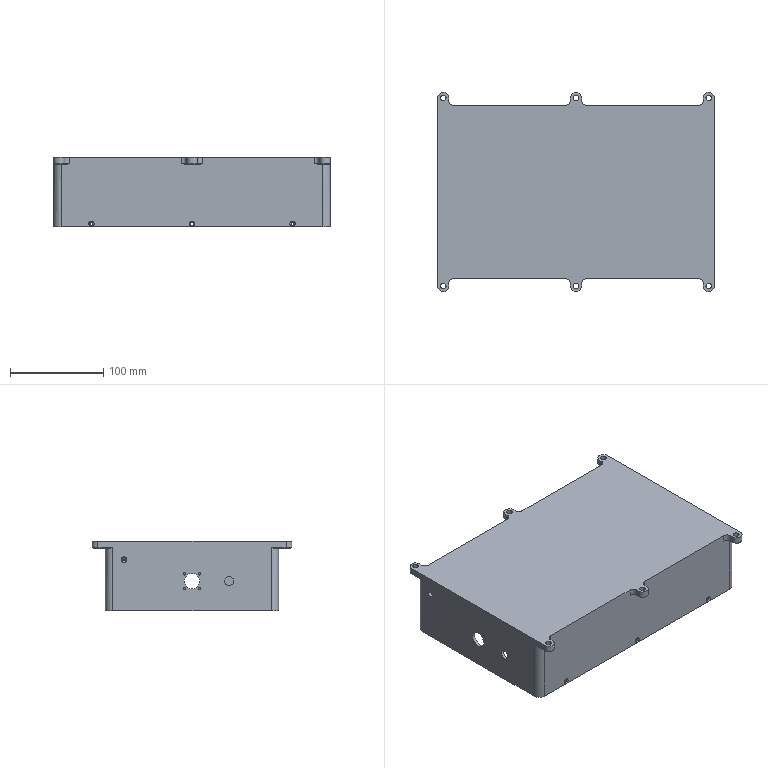NC program | NX | posted with a generic post | part box 297 x 214 x 75 mm
Whole program:
N10 G17 G21 G94 G90
(FLOOR_WALL_1_COPY_COPY , TOOL : D16)
N12 T02 M6
N14 G54
N16 G17 G0 G90 X-159.5 Y83.061 B0. C0. S7500 M3
N18 G43 Z30. H2
N20 Z-65.5
N22 G94 G1 Z-67. F1000.
N24 X-157.338 Y84.209
N26 G3 X-156.49 Y85.566 R1.6
N28 G2 X-140.5 Y101. R16.
N30 G1 X-128.5
N32 G3 X-127.114 Y101.8 R1.6
N34 G1 X-125.844 Y104.
N36 Z-65.5
N38 G0 Z30.
N40 X-16.656
N42 Z-65.5
N44 G1 Z-67.
N46 X-15.386 Y101.8
N48 G3 X-14. Y101. R1.6
N50 G1 X14.
N52 G3 X15.386 Y101.8 R1.6
N54 G1 X16.656 Y104.
N56 Z-65.5
N58 G0 Z30.
N60 X125.844
N62 Z-65.5
N64 G1 Z-67.
N66 X127.114 Y101.8
N68 G3 X128.5 Y101. R1.6
N70 G1 X140.5
N72 G2 X156.49 Y85.566 R16.
N74 G3 X157.338 Y84.209 R1.6
N76 G1 X159.5 Y83.061
N78 Z-65.5
N80 G0 Z30.
N82 Y-83.061
N84 Z-65.5
N86 G1 Z-67.
N88 X157.338 Y-84.209
N90 G3 X156.49 Y-85.566 R1.6
N92 G2 X140.5 Y-101. R16.
N94 G1 X128.5
N96 G3 X127.114 Y-101.8 R1.6
N98 G1 X125.844 Y-104.
N100 Z-65.5
N102 G0 Z30.
N104 X16.656
N106 Z-65.5
N108 G1 Z-67.
N110 X15.386 Y-101.8
N112 G3 X14. Y-101. R1.6
N114 G1 X-14.
N116 G3 X-15.386 Y-101.8 R1.6
N118 G1 X-16.656 Y-104.
N120 Z-65.5
N122 G0 Z30.
N124 X-125.844
N126 Z-65.5
N128 G1 Z-67.
N130 X-127.114 Y-101.8
N132 G3 X-128.5 Y-101. R1.6
N134 G1 X-140.5
N136 G2 X-156.49 Y-85.566 R16.
N138 G3 X-157.338 Y-84.209 R1.6
N140 G1 X-159.5 Y-83.061
N142 Z-65.5
N144 G0 Z30.
(ZLEVEL_PROFILE_1_COPY , TOOL : D10JING)
N146 T14 M6
N148 G17 G43 G0 G90 X138.036 Y83. Z30. B0. C0. S7500 H14 M3
N150 Z-13.633
N152 G94 G1 Z-16.633 F1000.
N154 X140. Y84.134
N156 G3 X140.5 Y85. R1.
N158 G1 X-140.5
N160 Y-85.
N162 X140.5
N164 Y85.
N166 G3 X139.634 Y84.5 R1.
N168 G1 X138.5 Y82.536
N170 Z-13.633
N172 G0 X138.036 Y83. Z-30.267
N174 G1 Z-33.267
N176 X140. Y84.134
N178 G3 X140.5 Y85. R1.
N180 G1 X-140.5
N182 Y-85.
N184 X140.5
N186 Y85.
N188 G3 X139.634 Y84.5 R1.
N190 G1 X138.5 Y82.536
N192 Z-30.267
N194 G0 X138.036 Y83. Z-46.9
N196 G1 Z-49.9
N198 X140. Y84.134
N200 G3 X140.5 Y85. R1.
N202 G1 X-140.5
N204 Y-85.
N206 X140.5
N208 Y85.
N210 G3 X139.634 Y84.5 R1.
N212 G1 X138.5 Y82.536
N214 Z-46.9
N216 G0 Z30.
N218 M5
N220 M2